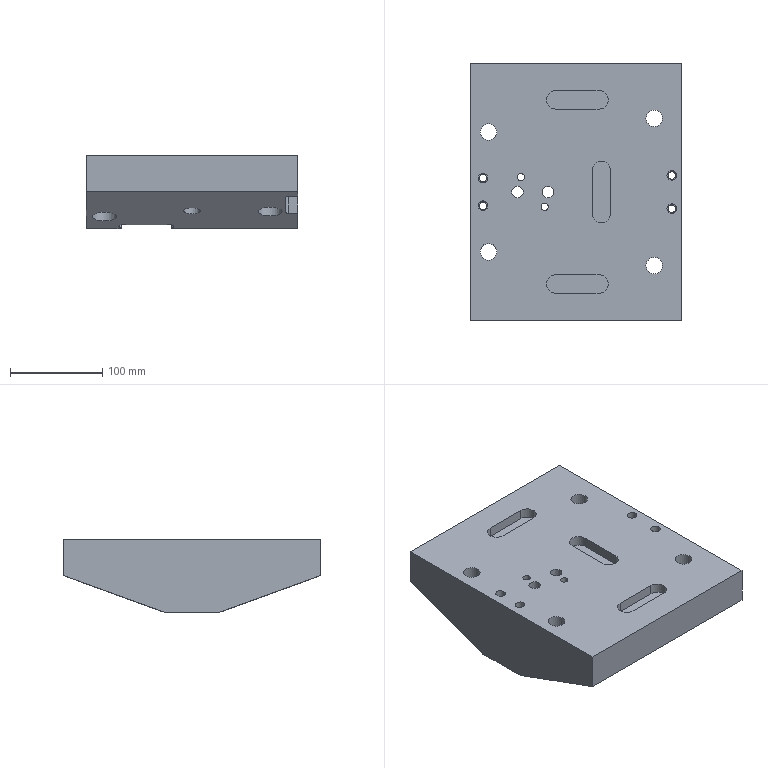Part | STEP file | lll_id3426_x_t | 1 solid | 101 faces | box 230 x 280 x 80 mm | volume 3699783 mm3 | cylinder 50 | plane 45 | cone 6 | commonest cylinder face diameters 20 x10 10 x8 8 x6 6 x4 10.5 x4 18.009 x4